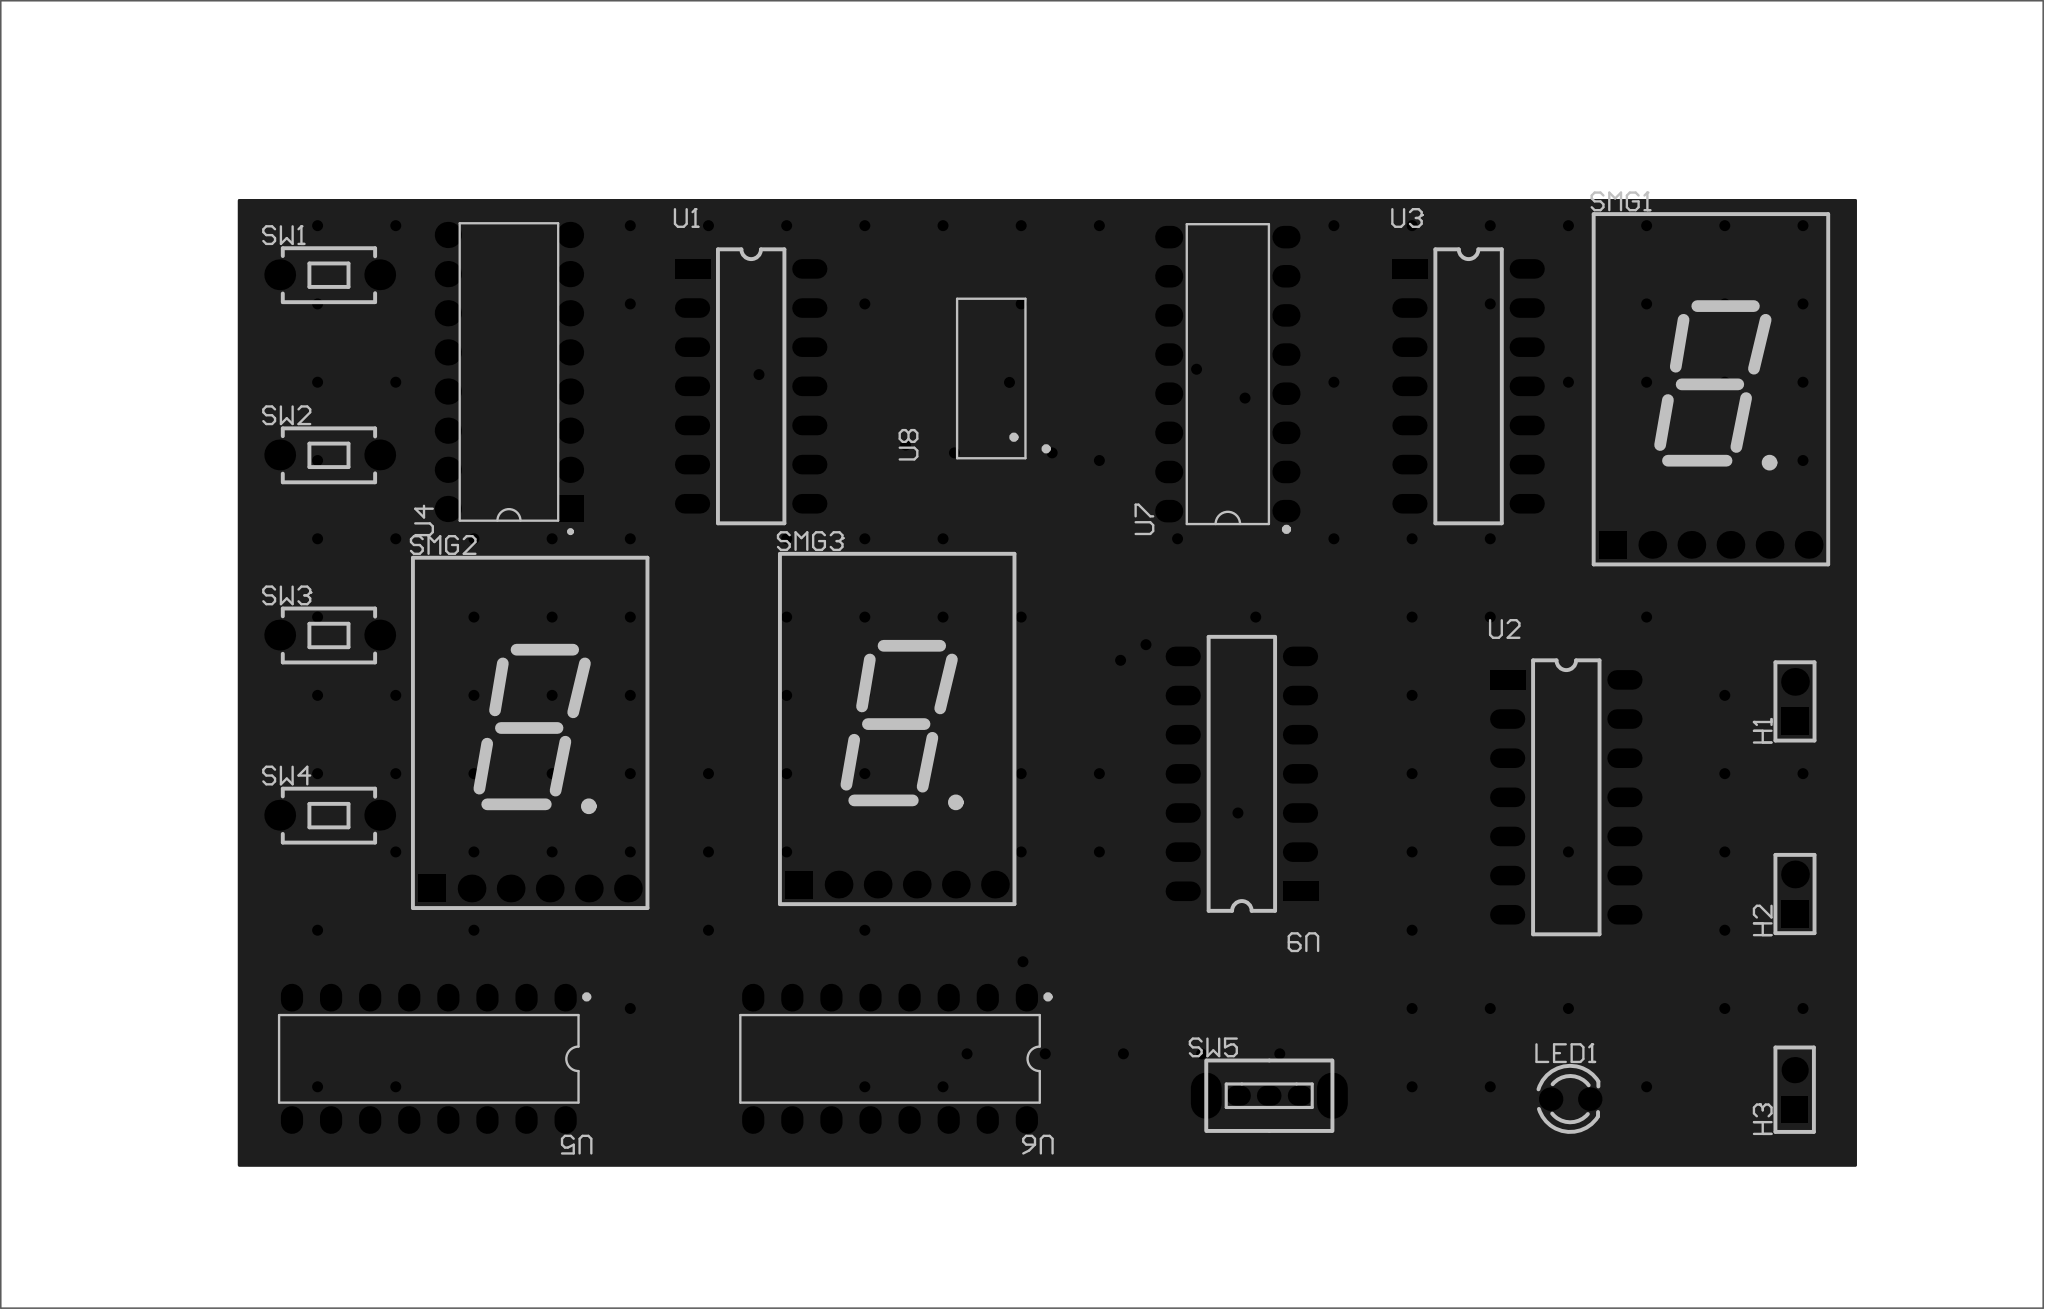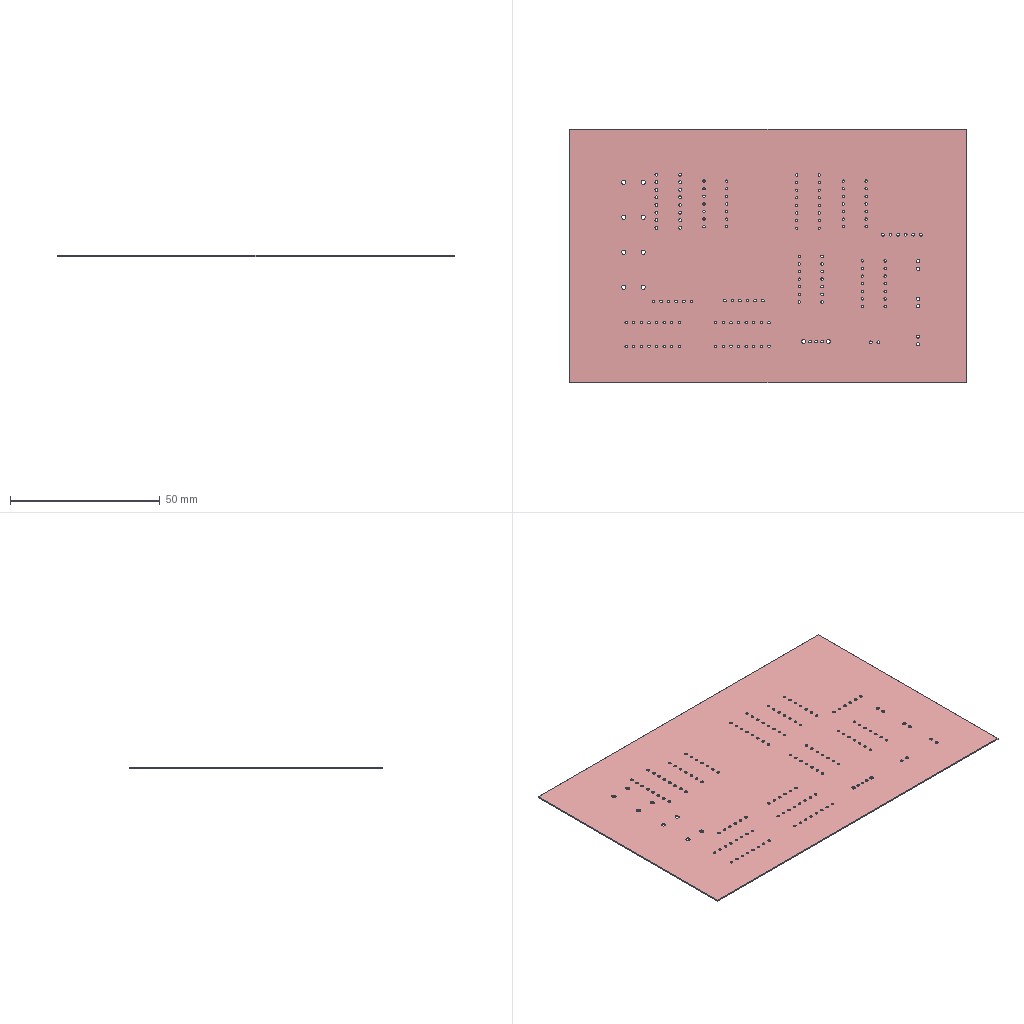Circuit board layout | Altium Designer | box 132.7 x 84.8 x 0.4 mm
Layer stack:
# Altium Designer layer stack of  (unit mm; dielectric type: 0 none, 1 core, 2 prepreg, 3 surface material)
index,name,kind,layer,copper_thickness_mm,dielectric_type,dielectric_thickness_mm,dielectric_material,dielectric_constant
0,Top Paste Mask Layer,other,,,,,,
1,Top Silkscreen Layer,other,,,,,,
2,Top Solder Mask Layer,dielectric,,,3,0.0102,Solder Resist,3.5
3,Top Layer,copper,Top Layer,0.0356,,,,
4,Dielectric 1,dielectric,,,3,0.32,FR-4,4.8
5,Bottom Layer,copper,Bottom Layer,0.0356,,,,
6,Bottom Solder Mask Layer,dielectric,,,3,0.0102,Solder Resist,3.5
7,Bottom Silkscreen Layer,other,,,,,,
8,Bottom Paste Mask Layer,other,,,,,,
# drill layer pairs: low layer,high layer
drill_pair,Top Layer,Bottom Layer
Part placement:
Designator,Comment,Layer,Footprint,Center-X(mm),Center-Y(mm),Rotation
H1,,TopLayer,HDR-TH_2P-P2.54-V-M-1,186.436,109.22,90
H2,,TopLayer,HDR-TH_2P-P2.54-V-M-1,186.436,96.722,90
H3,,TopLayer,HDR-TH_2P-P2.54-V-F,186.416,84.025,90
LED1,,TopLayer,LED_TH-3mm,171.831,83.413,0
SMG1,SMG,TopLayer,B含CD译码器的数码管,180.975,119.38,0
SMG2,SMG,TopLayer,B含CD译码器的数码管,104.251,97.082,0
SMG3,SMG,TopLayer,B含CD译码器的数码管,128.099,97.336,0
SW1,,TopLayer,Key_TH_3.5x6x4.3,91.224,136.906,0
SW2,,TopLayer,Key_TH_3.5x6x4.3,91.224,125.217,0
SW3,,TopLayer,Key_TH_3.5x6x4.3,91.224,113.527,0
SW4,,TopLayer,Key_TH_3.5x6x4.3,91.224,101.838,0
SW5,,TopLayer,拨动开关,152.281,83.634,0
U1,74LS04,TopLayer,DIP-014,118.611,129.667,0
U2,74LS32,TopLayer,DIP-014,171.577,102.997,0
U3,74LS00,TopLayer,DIP-014,165.227,129.667,0
U4,SN74148N,TopLayer,PDIP-16_L19.3-W6.4-P2.54-LS7.9-BL,102.87,130.599,90
U5,SN74LS192N(XBLW),TopLayer,PDIP-16_L19.3-W6.4-P2.54-LS7.94-BL,97.663,86.028,180
U6,SN74LS192N(XBLW),TopLayer,PDIP-16_L19.3-W6.4-P2.54-LS7.94-BL,127.635,86.028,180
U7,SN74175N,TopLayer,DIP-16_L19.3-W6.4-P2.54-LS7.6-BL,149.584,130.459,90
U8,SN74LS21NS,TopLayer,SOIC-14_L10.0-W5.5-P1.27-LS7.8-BL,134.213,130.175,90
U9,74LS04,TopLayer,DIP-014,150.495,104.521,180
Pad and via stacks:
# Altium Designer via and pad stacks of  (unit mm). Each distinct definition once, with the count of objects using it.
# via: kind,start_layer,end_layer,hole_mm,diameter_mm,mode(0 simple;1 top-mid-bottom;2 full stack),diameter_per_layer,count,example_net
# pad: kind,layer,hole_mm,hole_type(0 round;1 square;2 slot),plating,top_size,top_shape(1 round;2 rect;3 octagon;9 rounded rect),mid_size,bottom_size,mode,footprint,size_per_layer,count,example
pad,Multi-Layer,1.1,0,plated,1.8x1.8,1,1.8x1.8,1.8x1.8,0,HDR-TH_2P-P2.54-V-M-1,,2,H1.2
pad,Multi-Layer,1.1,0,plated,1.8x1.8,2,1.8x1.8,1.8x1.8,0,HDR-TH_2P-P2.54-V-M-1,,2,H1.1
pad,Multi-Layer,1,0,plated,1.7x1.7,2,1.7x1.7,1.7x1.7,0,HDR-TH_2P-P2.54-V-F,,1,H3.1
pad,Multi-Layer,1,0,plated,1.7x1.7,1,1.7x1.7,1.7x1.7,0,HDR-TH_2P-P2.54-V-F,,1,H3.2
pad,Multi-Layer,0.9144,0,plated,1.524x1.524,1,1.524x1.524,1.524x1.524,0,LED_TH-3mm,,2,LED1.1
pad,Multi-Layer,0.9,0,plated,1.8x1.8,1,1.8x1.8,1.8x1.8,0,B\u00BA\u00ACCD\u00D2\u00EB\u00C2\u00EB\u00C6\u00F7\u00B5\u00C4\u00CA\u00FD\u00C2\u00EB\u00B9\u00DC,,15,SMG1.6
pad,Multi-Layer,0.9,0,plated,1.8x1.8,2,1.8x1.8,1.8x1.8,0,B\u00BA\u00ACCD\u00D2\u00EB\u00C2\u00EB\u00C6\u00F7\u00B5\u00C4\u00CA\u00FD\u00C2\u00EB\u00B9\u00DC,,3,SMG1.1
pad,Multi-Layer,1.399,0,plated,1.999x1.999,1,1.999x1.999,1.999x1.999,0,Key_TH_3.5x6x4.3,,8,SW1.A
pad,Multi-Layer,0.8992,0,plated,1.6x1.3,1,1.6x1.3,1.6x1.3,0,\u00B2\u00A6\u00B6\u00AF\u00BF\u00AA\u00B9\u00D8,,3,SW5.1
pad,Multi-Layer,1.3,0,plated,3x1.999,1,3x1.999,3x1.999,0,\u00B2\u00A6\u00B6\u00AF\u00BF\u00AA\u00B9\u00D8,,2,SW5.4
pad,Multi-Layer,0.8128,0,plated,2.286x1.27,1,2.286x1.27,2.286x1.27,0,DIP-014,,52,U1.8
pad,Multi-Layer,0.8128,0,plated,2.286x1.27,2,2.286x1.27,2.286x1.27,0,DIP-014,,4,U1.1
pad,Multi-Layer,1,0,plated,1.7x1.7,2,1.7x1.7,1.7x1.7,0,PDIP-16_L19.3-W6.4-P2.54-LS7.9-BL,,1,U4.1
pad,Multi-Layer,1,0,plated,1.7x1.7,1,1.7x1.7,1.7x1.7,0,PDIP-16_L19.3-W6.4-P2.54-LS7.9-BL,,15,U4.2
pad,Multi-Layer,0.8,0,plated,1.44x1.8,1,1.44x1.8,1.44x1.8,0,PDIP-16_L19.3-W6.4-P2.54-LS7.94-BL,,32,U5.1
pad,Multi-Layer,0.8,0,plated,1.46x1.825,1,1.46x1.825,1.46x1.825,0,DIP-16_L19.3-W6.4-P2.54-LS7.6-BL,,16,U7.9
pad,Top Layer,0,0,plated,0.602x2.231,1,0.602x2.231,0.602x2.231,0,SOIC-14_L10.0-W5.5-P1.27-LS7.8-BL,,14,U8.1
via,Top Layer,Bottom Layer,0.3556,0.7112,0,,128,$1N837
Copper pours:
name,layer,net,type(0 solid;1 hatched;2 none)
Top Layer-GND,Top Layer,GND,0
Bottom Layer-GND,Bottom Layer,GND,0
Design rules, without the lines most boards share:
# Altium Designer design rules of  (exported by Altium Designer, unit mm)
# columns: name | kind | enabled | priority | scope1 | scope2 | descriptor | typed fields (field=value)
Plane_PlaneConnect | 0 | disabled | 1 | All | All | Clearance Constraint (Gap=10mil) (Disabled)(All),(All) | gap=0.254
Plane_PlaneConnect_1 | 63 | disabled | 1 | All | All | Board Clearance Constraint (Gap=0mil) (Disabled)(All) |
Copper_PolygonConnect | 0 | disabled | 2 | All | All | Clearance Constraint (Gap=10mil) (Disabled)(All),(All) | gap=0.254
Copper_PolygonConnect_1 | 63 | disabled | 2 | All | All | Board Clearance Constraint (Gap=0mil) (Disabled)(All) |
Clearance | 0 | enabled | 3 | All | All | Clearance Constraint (Gap=10mil) (All),(All) | gap=0.254
Clearance_1 | 63 | enabled | 3 | All | All | Board Clearance Constraint (Gap=0mil) (All) |
HoleToHoleClearance | 52 | enabled | 1 | All | All | Hole To Hole Clearance (Gap=10mil) (All),(All) | gap=0.254
Width | 2 | enabled | 1 | All | All | Width Constraint (Min=10mil) (Max=30mil) (Preferred=10mil) (All) |
DiffPairsRouting | 51 | enabled | 1 | All | All | Differential Pairs Uncoupled Length using the Gap Constraints (Min=10mil) (Max=10mil) (Prefered=10mil)  and Width Constraints (Min=15mil) (Max=15mil) (Prefered=15mil) (All) |
RoutingVias | 11 | enabled | 1 | All | All | Routing Via (MinHoleWidth=1mil) (MaxHoleWidth=28mil) (PreferredHoleWidth=28mil) (MinWidth=1mil) (MaxWidth=50mil) (PreferedWidth=50mil) (All) | via_min_hole=0.0254 via_max_hole=0.7112 via_preferred_diameter=1.27 via_preferred_hole=0.7112
PlaneConnect | 6 | enabled | 1 | All | All | Power Plane Connect Rule(Relief Connect )(Expansion=20mil) (Conductor Width=10mil) (Air Gap=10mil) (Entries=4) (All) | relief_conductor_width=0.254 relief_entries=4 relief_expansion=0.508
PolygonConnect | 20 | enabled | 1 | All | All | Polygon Connect Rule(Relief Connect )(Conductor Width=0mil) (Relief Angle=90 Angle) (Entries=4) (Air Gap Width=1mil) (All),(All) | connect_style(0=relief,1=direct,2=none)=0 relief_conductor_width=0 relief_entries=4
PasteMaskExpansion | 14 | enabled | 1 | All | All | Paste Mask Expansion (Expansion =0mil) (All) | expansion=0
SolderMaskExpansion | 13 | enabled | 1 | All | All | Solder Mask Expansion (Expansion =4mil) (All) | expansion=0.1016